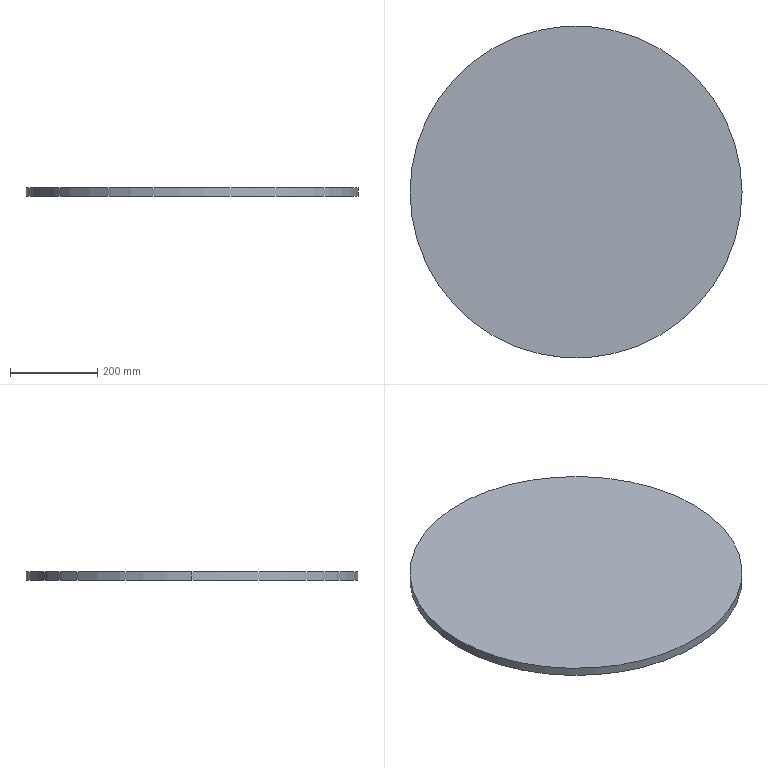Part | SolidWorks | features Extrusion 1 | 1 solid | 4 faces | box 760 x 760 x 20 mm | volume 9072920 mm3 | cylinder 2 | plane 2 | commonest cylinder face diameters 760 x2
STEP:
#1=CARTESIAN_POINT('',(380.,0.,20.));
#2=VERTEX_POINT('',#1);
#3=CARTESIAN_POINT('',(-380.,0.,20.));
#4=VERTEX_POINT('',#3);
#5=CARTESIAN_POINT('',(0.,0.,20.));
#6=DIRECTION('',(0.,0.,1.));
#7=DIRECTION('',(1.,0.,0.));
#8=AXIS2_PLACEMENT_3D('',#5,#6,#7);
#9=CIRCLE('',#8,380.);
#10=EDGE_CURVE('',#2,#4,#9,.T.);
#11=ORIENTED_EDGE('',*,*,#10,.F.);
#12=CARTESIAN_POINT('',(380.,0.,0.));
#13=VERTEX_POINT('',#12);
#14=CARTESIAN_POINT('',(380.,0.,20.));
#15=DIRECTION('',(0.,0.,-1.));
#16=VECTOR('',#15,1000.);
#17=LINE('',#14,#16);
#18=EDGE_CURVE('',#2,#13,#17,.T.);
#19=ORIENTED_EDGE('',*,*,#18,.T.);
#20=CARTESIAN_POINT('',(-380.,0.,0.));
#21=VERTEX_POINT('',#20);
#22=CARTESIAN_POINT('',(0.,0.,0.));
#23=DIRECTION('',(0.,0.,1.));
#24=DIRECTION('',(1.,0.,0.));
#25=AXIS2_PLACEMENT_3D('',#22,#23,#24);
#26=CIRCLE('',#25,380.);
#27=EDGE_CURVE('',#13,#21,#26,.T.);
#28=ORIENTED_EDGE('',*,*,#27,.T.);
#29=CARTESIAN_POINT('',(-380.,0.,20.));
#30=DIRECTION('',(0.,0.,-1.));
#31=VECTOR('',#30,1000.);
#32=LINE('',#29,#31);
#33=EDGE_CURVE('',#4,#21,#32,.T.);
#34=ORIENTED_EDGE('',*,*,#33,.F.);
#35=EDGE_LOOP('',(#11,#19,#28,#34));
#36=FACE_OUTER_BOUND('',#35,.T.);
#37=CARTESIAN_POINT('',(0.,0.,20.));
#38=DIRECTION('',(0.,0.,-1.));
#39=DIRECTION('',(-1.,0.,0.));
#40=AXIS2_PLACEMENT_3D('',#37,#38,#39);
#41=CYLINDRICAL_SURFACE('',#40,380.);
#42=ADVANCED_FACE('',(#36),#41,.T.);
#43=ORIENTED_EDGE('',*,*,#18,.F.);
#44=CARTESIAN_POINT('',(0.,0.,20.));
#45=DIRECTION('',(0.,0.,1.));
#46=DIRECTION('',(1.,0.,0.));
#47=AXIS2_PLACEMENT_3D('',#44,#45,#46);
#48=CIRCLE('',#47,380.);
#49=EDGE_CURVE('',#4,#2,#48,.T.);
#50=ORIENTED_EDGE('',*,*,#49,.F.);
#51=ORIENTED_EDGE('',*,*,#33,.T.);
#52=CARTESIAN_POINT('',(0.,0.,0.));
#53=DIRECTION('',(0.,0.,1.));
#54=DIRECTION('',(1.,0.,0.));
#55=AXIS2_PLACEMENT_3D('',#52,#53,#54);
#56=CIRCLE('',#55,380.);
#57=EDGE_CURVE('',#21,#13,#56,.T.);
#58=ORIENTED_EDGE('',*,*,#57,.T.);
#59=EDGE_LOOP('',(#43,#50,#51,#58));
#60=FACE_OUTER_BOUND('',#59,.T.);
#61=CARTESIAN_POINT('',(0.,0.,20.));
#62=DIRECTION('',(0.,0.,-1.));
#63=DIRECTION('',(-1.,0.,0.));
#64=AXIS2_PLACEMENT_3D('',#61,#62,#63);
#65=CYLINDRICAL_SURFACE('',#64,380.);
#66=ADVANCED_FACE('',(#60),#65,.T.);
#67=ORIENTED_EDGE('',*,*,#49,.T.);
#68=ORIENTED_EDGE('',*,*,#10,.T.);
#69=EDGE_LOOP('',(#67,#68));
#70=FACE_OUTER_BOUND('',#69,.T.);
#71=CARTESIAN_POINT('',(0.,0.,20.));
#72=DIRECTION('',(0.,0.,1.));
#73=DIRECTION('',(1.,0.,0.));
#74=AXIS2_PLACEMENT_3D('',#71,#72,#73);
#75=PLANE('',#74);
#76=ADVANCED_FACE('',(#70),#75,.T.);
#77=ORIENTED_EDGE('',*,*,#57,.F.);
#78=ORIENTED_EDGE('',*,*,#27,.F.);
#79=EDGE_LOOP('',(#77,#78));
#80=FACE_OUTER_BOUND('',#79,.T.);
#81=CARTESIAN_POINT('',(0.,0.,0.));
#82=DIRECTION('',(0.,0.,1.));
#83=DIRECTION('',(1.,0.,0.));
#84=AXIS2_PLACEMENT_3D('',#81,#82,#83);
#85=PLANE('',#84);
#86=ADVANCED_FACE('',(#80),#85,.F.);
#87=CLOSED_SHELL('',(#42,#66,#76,#86));
#88=MANIFOLD_SOLID_BREP('',#87);
#89=CARTESIAN_POINT('',(0.,0.,0.));
#90=DIRECTION('',(0.,0.,1.));
#91=DIRECTION('',(1.,0.,0.));
#92=AXIS2_PLACEMENT_3D('',#89,#90,#91);
#93=(LENGTH_UNIT()NAMED_UNIT(*)SI_UNIT(.MILLI.,.METRE.));
#94=UNCERTAINTY_MEASURE_WITH_UNIT(LENGTH_MEASURE(0.00001),#93,'','');
#95=(NAMED_UNIT(*)PLANE_ANGLE_UNIT()SI_UNIT($,.RADIAN.));
#96=(NAMED_UNIT(*)SI_UNIT($,.STERADIAN.)SOLID_ANGLE_UNIT());
#97=(GEOMETRIC_REPRESENTATION_CONTEXT(3)GLOBAL_UNCERTAINTY_ASSIGNED_CONTEXT((#94))GLOBAL_UNIT_ASSIGNED_CONTEXT((#93,#95,#96))REPRESENTATION_CONTEXT('',''));
#98=ADVANCED_BREP_SHAPE_REPRESENTATION('',(#88,#92),#97);